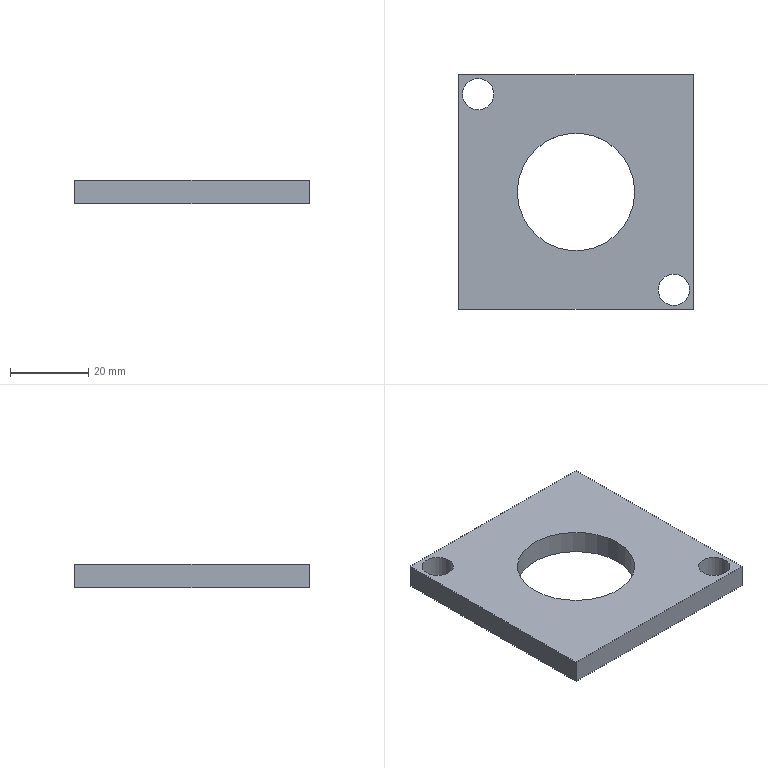Part | NX | features solid 2 | 1 solid | 9 faces | box 60 x 60 x 6 mm | volume 16756 mm3 | plane 6 | cylinder 3 | commonest cylinder face diameters 8 x2 30 x1
STEP:
#1=CARTESIAN_POINT('',(-100.,-185.,-131.));
#2=VERTEX_POINT('',#1);
#3=CARTESIAN_POINT('',(-100.,-125.,-131.));
#4=VERTEX_POINT('',#3);
#5=CARTESIAN_POINT('',(-100.,-185.,-131.));
#6=DIRECTION('',(0.,1.,0.));
#7=VECTOR('',#6,1000.);
#8=LINE('',#5,#7);
#9=EDGE_CURVE('',#2,#4,#8,.T.);
#10=ORIENTED_EDGE('',*,*,#9,.F.);
#11=CARTESIAN_POINT('',(-100.,-185.,-125.));
#12=VERTEX_POINT('',#11);
#13=CARTESIAN_POINT('',(-100.,-185.,-125.));
#14=DIRECTION('',(0.,0.,-1.));
#15=VECTOR('',#14,1000.);
#16=LINE('',#13,#15);
#17=EDGE_CURVE('',#12,#2,#16,.T.);
#18=ORIENTED_EDGE('',*,*,#17,.F.);
#19=CARTESIAN_POINT('',(-100.,-125.,-125.));
#20=VERTEX_POINT('',#19);
#21=CARTESIAN_POINT('',(-100.,-185.,-125.));
#22=DIRECTION('',(0.,1.,0.));
#23=VECTOR('',#22,1000.);
#24=LINE('',#21,#23);
#25=EDGE_CURVE('',#12,#20,#24,.T.);
#26=ORIENTED_EDGE('',*,*,#25,.T.);
#27=CARTESIAN_POINT('',(-100.,-125.,-125.));
#28=DIRECTION('',(0.,0.,-1.));
#29=VECTOR('',#28,1000.);
#30=LINE('',#27,#29);
#31=EDGE_CURVE('',#20,#4,#30,.T.);
#32=ORIENTED_EDGE('',*,*,#31,.T.);
#33=EDGE_LOOP('',(#10,#18,#26,#32));
#34=FACE_BOUND('',#33,.T.);
#35=CARTESIAN_POINT('',(-100.,-185.,-125.));
#36=DIRECTION('',(-1.,0.,0.));
#37=DIRECTION('',(0.,0.,1.));
#38=AXIS2_PLACEMENT_3D('',#35,#36,#37);
#39=PLANE('',#38);
#40=ADVANCED_FACE('',(#34),#39,.T.);
#41=CARTESIAN_POINT('',(-40.,-185.,-131.));
#42=VERTEX_POINT('',#41);
#43=CARTESIAN_POINT('',(-40.,-185.,-131.));
#44=DIRECTION('',(-1.,0.,0.));
#45=VECTOR('',#44,1000.);
#46=LINE('',#43,#45);
#47=EDGE_CURVE('',#42,#2,#46,.T.);
#48=ORIENTED_EDGE('',*,*,#47,.F.);
#49=CARTESIAN_POINT('',(-40.,-185.,-125.));
#50=VERTEX_POINT('',#49);
#51=CARTESIAN_POINT('',(-40.,-185.,-125.));
#52=DIRECTION('',(0.,0.,-1.));
#53=VECTOR('',#52,1000.);
#54=LINE('',#51,#53);
#55=EDGE_CURVE('',#50,#42,#54,.T.);
#56=ORIENTED_EDGE('',*,*,#55,.F.);
#57=CARTESIAN_POINT('',(-40.,-185.,-125.));
#58=DIRECTION('',(-1.,0.,0.));
#59=VECTOR('',#58,1000.);
#60=LINE('',#57,#59);
#61=EDGE_CURVE('',#50,#12,#60,.T.);
#62=ORIENTED_EDGE('',*,*,#61,.T.);
#63=ORIENTED_EDGE('',*,*,#17,.T.);
#64=EDGE_LOOP('',(#48,#56,#62,#63));
#65=FACE_BOUND('',#64,.T.);
#66=CARTESIAN_POINT('',(-40.,-185.,-125.));
#67=DIRECTION('',(0.,-1.,0.));
#68=DIRECTION('',(1.,0.,0.));
#69=AXIS2_PLACEMENT_3D('',#66,#67,#68);
#70=PLANE('',#69);
#71=ADVANCED_FACE('',(#65),#70,.T.);
#72=CARTESIAN_POINT('',(-40.,-125.,-131.));
#73=VERTEX_POINT('',#72);
#74=CARTESIAN_POINT('',(-40.,-125.,-131.));
#75=DIRECTION('',(0.,-1.,0.));
#76=VECTOR('',#75,1000.);
#77=LINE('',#74,#76);
#78=EDGE_CURVE('',#73,#42,#77,.T.);
#79=ORIENTED_EDGE('',*,*,#78,.F.);
#80=CARTESIAN_POINT('',(-40.,-125.,-125.));
#81=VERTEX_POINT('',#80);
#82=CARTESIAN_POINT('',(-40.,-125.,-125.));
#83=DIRECTION('',(0.,0.,-1.));
#84=VECTOR('',#83,1000.);
#85=LINE('',#82,#84);
#86=EDGE_CURVE('',#81,#73,#85,.T.);
#87=ORIENTED_EDGE('',*,*,#86,.F.);
#88=CARTESIAN_POINT('',(-40.,-125.,-125.));
#89=DIRECTION('',(0.,-1.,0.));
#90=VECTOR('',#89,1000.);
#91=LINE('',#88,#90);
#92=EDGE_CURVE('',#81,#50,#91,.T.);
#93=ORIENTED_EDGE('',*,*,#92,.T.);
#94=ORIENTED_EDGE('',*,*,#55,.T.);
#95=EDGE_LOOP('',(#79,#87,#93,#94));
#96=FACE_BOUND('',#95,.T.);
#97=CARTESIAN_POINT('',(-40.,-125.,-125.));
#98=DIRECTION('',(1.,0.,0.));
#99=DIRECTION('',(0.,0.,-1.));
#100=AXIS2_PLACEMENT_3D('',#97,#98,#99);
#101=PLANE('',#100);
#102=ADVANCED_FACE('',(#96),#101,.T.);
#103=CARTESIAN_POINT('',(-55.,-155.,-125.));
#104=VERTEX_POINT('',#103);
#105=CARTESIAN_POINT('',(-70.,-155.,-125.));
#106=DIRECTION('',(0.,0.,1.));
#107=DIRECTION('',(1.,0.,0.));
#108=AXIS2_PLACEMENT_3D('',#105,#106,#107);
#109=CIRCLE('',#108,15.);
#110=EDGE_CURVE('',#104,#104,#109,.T.);
#111=ORIENTED_EDGE('',*,*,#110,.T.);
#112=EDGE_LOOP('',(#111));
#113=FACE_BOUND('',#112,.T.);
#114=CARTESIAN_POINT('',(-55.,-155.,-131.));
#115=VERTEX_POINT('',#114);
#116=CARTESIAN_POINT('',(-70.,-155.,-131.));
#117=DIRECTION('',(0.,0.,1.));
#118=DIRECTION('',(1.,0.,0.));
#119=AXIS2_PLACEMENT_3D('',#116,#117,#118);
#120=CIRCLE('',#119,15.);
#121=EDGE_CURVE('',#115,#115,#120,.T.);
#122=ORIENTED_EDGE('',*,*,#121,.F.);
#123=EDGE_LOOP('',(#122));
#124=FACE_BOUND('',#123,.T.);
#125=CARTESIAN_POINT('',(-70.,-155.,-125.));
#126=DIRECTION('',(0.,0.,-1.));
#127=DIRECTION('',(-1.,0.,0.));
#128=AXIS2_PLACEMENT_3D('',#125,#126,#127);
#129=CYLINDRICAL_SURFACE('',#128,15.);
#130=ADVANCED_FACE('',(#113,#124),#129,.F.);
#131=CARTESIAN_POINT('',(-41.,-180.,-125.));
#132=VERTEX_POINT('',#131);
#133=CARTESIAN_POINT('',(-45.,-180.,-125.));
#134=DIRECTION('',(0.,0.,1.));
#135=DIRECTION('',(1.,0.,0.));
#136=AXIS2_PLACEMENT_3D('',#133,#134,#135);
#137=CIRCLE('',#136,4.);
#138=EDGE_CURVE('',#132,#132,#137,.T.);
#139=ORIENTED_EDGE('',*,*,#138,.T.);
#140=EDGE_LOOP('',(#139));
#141=FACE_BOUND('',#140,.T.);
#142=CARTESIAN_POINT('',(-41.,-180.,-131.));
#143=VERTEX_POINT('',#142);
#144=CARTESIAN_POINT('',(-45.,-180.,-131.));
#145=DIRECTION('',(0.,0.,1.));
#146=DIRECTION('',(1.,0.,0.));
#147=AXIS2_PLACEMENT_3D('',#144,#145,#146);
#148=CIRCLE('',#147,4.);
#149=EDGE_CURVE('',#143,#143,#148,.T.);
#150=ORIENTED_EDGE('',*,*,#149,.F.);
#151=EDGE_LOOP('',(#150));
#152=FACE_BOUND('',#151,.T.);
#153=CARTESIAN_POINT('',(-45.,-180.,-125.));
#154=DIRECTION('',(0.,0.,-1.));
#155=DIRECTION('',(-1.,0.,0.));
#156=AXIS2_PLACEMENT_3D('',#153,#154,#155);
#157=CYLINDRICAL_SURFACE('',#156,4.);
#158=ADVANCED_FACE('',(#141,#152),#157,.F.);
#159=CARTESIAN_POINT('',(-91.,-130.,-125.));
#160=VERTEX_POINT('',#159);
#161=CARTESIAN_POINT('',(-95.,-130.,-125.));
#162=DIRECTION('',(0.,0.,1.));
#163=DIRECTION('',(1.,0.,0.));
#164=AXIS2_PLACEMENT_3D('',#161,#162,#163);
#165=CIRCLE('',#164,4.);
#166=EDGE_CURVE('',#160,#160,#165,.T.);
#167=ORIENTED_EDGE('',*,*,#166,.T.);
#168=EDGE_LOOP('',(#167));
#169=FACE_BOUND('',#168,.T.);
#170=CARTESIAN_POINT('',(-91.,-130.,-131.));
#171=VERTEX_POINT('',#170);
#172=CARTESIAN_POINT('',(-95.,-130.,-131.));
#173=DIRECTION('',(0.,0.,1.));
#174=DIRECTION('',(1.,0.,0.));
#175=AXIS2_PLACEMENT_3D('',#172,#173,#174);
#176=CIRCLE('',#175,4.);
#177=EDGE_CURVE('',#171,#171,#176,.T.);
#178=ORIENTED_EDGE('',*,*,#177,.F.);
#179=EDGE_LOOP('',(#178));
#180=FACE_BOUND('',#179,.T.);
#181=CARTESIAN_POINT('',(-95.,-130.,-125.));
#182=DIRECTION('',(0.,0.,-1.));
#183=DIRECTION('',(-1.,0.,0.));
#184=AXIS2_PLACEMENT_3D('',#181,#182,#183);
#185=CYLINDRICAL_SURFACE('',#184,4.);
#186=ADVANCED_FACE('',(#169,#180),#185,.F.);
#187=CARTESIAN_POINT('',(-100.,-125.,-131.));
#188=DIRECTION('',(1.,0.,0.));
#189=VECTOR('',#188,1000.);
#190=LINE('',#187,#189);
#191=EDGE_CURVE('',#4,#73,#190,.T.);
#192=ORIENTED_EDGE('',*,*,#191,.F.);
#193=ORIENTED_EDGE('',*,*,#31,.F.);
#194=CARTESIAN_POINT('',(-100.,-125.,-125.));
#195=DIRECTION('',(1.,0.,0.));
#196=VECTOR('',#195,1000.);
#197=LINE('',#194,#196);
#198=EDGE_CURVE('',#20,#81,#197,.T.);
#199=ORIENTED_EDGE('',*,*,#198,.T.);
#200=ORIENTED_EDGE('',*,*,#86,.T.);
#201=EDGE_LOOP('',(#192,#193,#199,#200));
#202=FACE_BOUND('',#201,.T.);
#203=CARTESIAN_POINT('',(-100.,-125.,-125.));
#204=DIRECTION('',(0.,1.,0.));
#205=DIRECTION('',(0.,0.,1.));
#206=AXIS2_PLACEMENT_3D('',#203,#204,#205);
#207=PLANE('',#206);
#208=ADVANCED_FACE('',(#202),#207,.T.);
#209=ORIENTED_EDGE('',*,*,#166,.F.);
#210=EDGE_LOOP('',(#209));
#211=FACE_BOUND('',#210,.T.);
#212=ORIENTED_EDGE('',*,*,#138,.F.);
#213=EDGE_LOOP('',(#212));
#214=FACE_BOUND('',#213,.T.);
#215=ORIENTED_EDGE('',*,*,#110,.F.);
#216=EDGE_LOOP('',(#215));
#217=FACE_BOUND('',#216,.T.);
#218=ORIENTED_EDGE('',*,*,#198,.F.);
#219=ORIENTED_EDGE('',*,*,#25,.F.);
#220=ORIENTED_EDGE('',*,*,#61,.F.);
#221=ORIENTED_EDGE('',*,*,#92,.F.);
#222=EDGE_LOOP('',(#218,#219,#220,#221));
#223=FACE_BOUND('',#222,.T.);
#224=CARTESIAN_POINT('',(-100.,-185.,-125.));
#225=DIRECTION('',(0.,0.,1.));
#226=DIRECTION('',(1.,0.,0.));
#227=AXIS2_PLACEMENT_3D('',#224,#225,#226);
#228=PLANE('',#227);
#229=ADVANCED_FACE('',(#211,#214,#217,#223),#228,.T.);
#230=ORIENTED_EDGE('',*,*,#177,.T.);
#231=EDGE_LOOP('',(#230));
#232=FACE_BOUND('',#231,.T.);
#233=ORIENTED_EDGE('',*,*,#149,.T.);
#234=EDGE_LOOP('',(#233));
#235=FACE_BOUND('',#234,.T.);
#236=ORIENTED_EDGE('',*,*,#121,.T.);
#237=EDGE_LOOP('',(#236));
#238=FACE_BOUND('',#237,.T.);
#239=ORIENTED_EDGE('',*,*,#9,.T.);
#240=ORIENTED_EDGE('',*,*,#191,.T.);
#241=ORIENTED_EDGE('',*,*,#78,.T.);
#242=ORIENTED_EDGE('',*,*,#47,.T.);
#243=EDGE_LOOP('',(#239,#240,#241,#242));
#244=FACE_BOUND('',#243,.T.);
#245=CARTESIAN_POINT('',(-100.,-185.,-131.));
#246=DIRECTION('',(0.,0.,1.));
#247=DIRECTION('',(1.,0.,0.));
#248=AXIS2_PLACEMENT_3D('',#245,#246,#247);
#249=PLANE('',#248);
#250=ADVANCED_FACE('',(#232,#235,#238,#244),#249,.F.);
#251=CLOSED_SHELL('',(#40,#71,#102,#130,#158,#186,#208,#229,#250));
#252=MANIFOLD_SOLID_BREP('',#251);
#253=(LENGTH_UNIT()NAMED_UNIT(*)SI_UNIT(.MILLI.,.METRE.));
#254=UNCERTAINTY_MEASURE_WITH_UNIT(LENGTH_MEASURE(0.00001),#253,'','');
#255=(NAMED_UNIT(*)PLANE_ANGLE_UNIT()SI_UNIT($,.RADIAN.));
#256=(NAMED_UNIT(*)SI_UNIT($,.STERADIAN.)SOLID_ANGLE_UNIT());
#257=(GEOMETRIC_REPRESENTATION_CONTEXT(3)GLOBAL_UNCERTAINTY_ASSIGNED_CONTEXT((#254))GLOBAL_UNIT_ASSIGNED_CONTEXT((#253,#255,#256))REPRESENTATION_CONTEXT('',''));
#258=ADVANCED_BREP_SHAPE_REPRESENTATION('',(#252),#257);